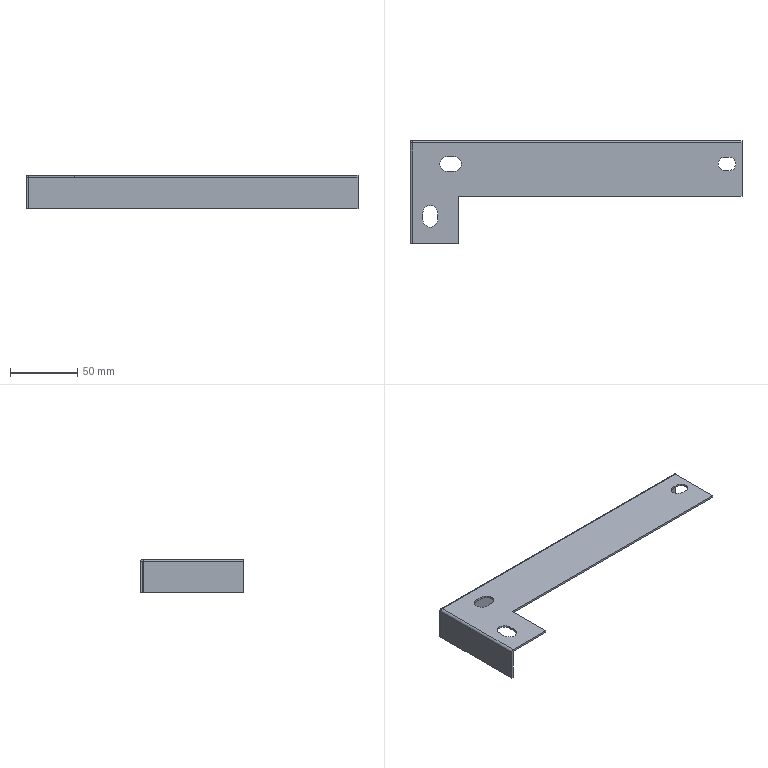Part | SolidWorks | features MirrorStock 1 | 1 solid | 39 faces | box 246 x 76 x 25 mm | volume 27497 mm3 | plane 27 | cylinder 12 | commonest cylinder face diameters 11 x5 10 x3 0.4 x2 3.4 x2
STEP:
#1=CARTESIAN_POINT('',(113.3,15.8,1.5));
#2=VERTEX_POINT('',#1);
#3=CARTESIAN_POINT('',(118.3,20.8,1.5));
#4=VERTEX_POINT('',#3);
#5=CARTESIAN_POINT('',(113.3,20.8,1.5));
#6=DIRECTION('',(0.,0.,1.));
#7=DIRECTION('',(1.,0.,0.));
#8=AXIS2_PLACEMENT_3D('',#5,#6,#7);
#9=CIRCLE('',#8,5.);
#10=EDGE_CURVE('',#2,#4,#9,.T.);
#11=ORIENTED_EDGE('',*,*,#10,.T.);
#12=CARTESIAN_POINT('',(118.3,20.8,0.));
#13=VERTEX_POINT('',#12);
#14=CARTESIAN_POINT('',(118.3,20.8,10.));
#15=DIRECTION('',(0.,0.,-1.));
#16=VECTOR('',#15,1000.);
#17=LINE('',#14,#16);
#18=EDGE_CURVE('',#4,#13,#17,.T.);
#19=ORIENTED_EDGE('',*,*,#18,.T.);
#20=CARTESIAN_POINT('',(113.3,15.8,0.));
#21=VERTEX_POINT('',#20);
#22=CARTESIAN_POINT('',(113.3,20.8,0.));
#23=DIRECTION('',(0.,0.,1.));
#24=DIRECTION('',(1.,0.,0.));
#25=AXIS2_PLACEMENT_3D('',#22,#23,#24);
#26=CIRCLE('',#25,5.);
#27=EDGE_CURVE('',#21,#13,#26,.T.);
#28=ORIENTED_EDGE('',*,*,#27,.F.);
#29=CARTESIAN_POINT('',(113.3,15.8,10.));
#30=DIRECTION('',(0.,0.,-1.));
#31=VECTOR('',#30,1000.);
#32=LINE('',#29,#31);
#33=EDGE_CURVE('',#2,#21,#32,.T.);
#34=ORIENTED_EDGE('',*,*,#33,.F.);
#35=EDGE_LOOP('',(#11,#19,#28,#34));
#36=FACE_OUTER_BOUND('',#35,.T.);
#37=CARTESIAN_POINT('',(113.3,20.8,10.));
#38=DIRECTION('',(0.,0.,-1.));
#39=DIRECTION('',(1.,0.,0.));
#40=AXIS2_PLACEMENT_3D('',#37,#38,#39);
#41=CYLINDRICAL_SURFACE('',#40,5.);
#42=ADVANCED_FACE('',(#36),#41,.F.);
#43=CARTESIAN_POINT('',(-90.5,15.3,1.5));
#44=VERTEX_POINT('',#43);
#45=CARTESIAN_POINT('',(-85.,20.8,1.5));
#46=VERTEX_POINT('',#45);
#47=CARTESIAN_POINT('',(-90.5,20.8,1.5));
#48=DIRECTION('',(0.,0.,1.));
#49=DIRECTION('',(1.,0.,0.));
#50=AXIS2_PLACEMENT_3D('',#47,#48,#49);
#51=CIRCLE('',#50,5.5);
#52=EDGE_CURVE('',#44,#46,#51,.T.);
#53=ORIENTED_EDGE('',*,*,#52,.T.);
#54=CARTESIAN_POINT('',(-85.,20.8,0.));
#55=VERTEX_POINT('',#54);
#56=CARTESIAN_POINT('',(-85.,20.8,10.));
#57=DIRECTION('',(0.,0.,-1.));
#58=VECTOR('',#57,1000.);
#59=LINE('',#56,#58);
#60=EDGE_CURVE('',#46,#55,#59,.T.);
#61=ORIENTED_EDGE('',*,*,#60,.T.);
#62=CARTESIAN_POINT('',(-90.5,15.3,0.));
#63=VERTEX_POINT('',#62);
#64=CARTESIAN_POINT('',(-90.5,20.8,0.));
#65=DIRECTION('',(0.,0.,1.));
#66=DIRECTION('',(1.,0.,0.));
#67=AXIS2_PLACEMENT_3D('',#64,#65,#66);
#68=CIRCLE('',#67,5.5);
#69=EDGE_CURVE('',#63,#55,#68,.T.);
#70=ORIENTED_EDGE('',*,*,#69,.F.);
#71=CARTESIAN_POINT('',(-90.5,15.3,10.));
#72=DIRECTION('',(0.,0.,-1.));
#73=VECTOR('',#72,1000.);
#74=LINE('',#71,#73);
#75=EDGE_CURVE('',#44,#63,#74,.T.);
#76=ORIENTED_EDGE('',*,*,#75,.F.);
#77=EDGE_LOOP('',(#53,#61,#70,#76));
#78=FACE_OUTER_BOUND('',#77,.T.);
#79=CARTESIAN_POINT('',(-90.5,20.8,10.));
#80=DIRECTION('',(0.,0.,-1.));
#81=DIRECTION('',(1.,0.,0.));
#82=AXIS2_PLACEMENT_3D('',#79,#80,#81);
#83=CYLINDRICAL_SURFACE('',#82,5.5);
#84=ADVANCED_FACE('',(#78),#83,.F.);
#85=CARTESIAN_POINT('',(-121.3,36.5,-0.2));
#86=VERTEX_POINT('',#85);
#87=CARTESIAN_POINT('',(-121.3,38.,-0.2));
#88=VERTEX_POINT('',#87);
#89=CARTESIAN_POINT('',(-121.3,36.5,-0.2));
#90=DIRECTION('',(0.,1.,0.));
#91=VECTOR('',#90,1000.);
#92=LINE('',#89,#91);
#93=EDGE_CURVE('',#86,#88,#92,.T.);
#94=ORIENTED_EDGE('',*,*,#93,.T.);
#95=CARTESIAN_POINT('',(-123.,38.,-0.2));
#96=VERTEX_POINT('',#95);
#97=CARTESIAN_POINT('',(123.,38.,-0.2));
#98=DIRECTION('',(1.,0.,0.));
#99=VECTOR('',#98,1000.);
#100=LINE('',#97,#99);
#101=EDGE_CURVE('',#96,#88,#100,.T.);
#102=ORIENTED_EDGE('',*,*,#101,.F.);
#103=CARTESIAN_POINT('',(-123.,36.5,-0.2));
#104=VERTEX_POINT('',#103);
#105=CARTESIAN_POINT('',(-123.,36.5,-0.2));
#106=DIRECTION('',(0.,1.,0.));
#107=VECTOR('',#106,1000.);
#108=LINE('',#105,#107);
#109=EDGE_CURVE('',#104,#96,#108,.T.);
#110=ORIENTED_EDGE('',*,*,#109,.F.);
#111=CARTESIAN_POINT('',(123.,36.5,-0.2));
#112=DIRECTION('',(-1.,0.,0.));
#113=VECTOR('',#112,1000.);
#114=LINE('',#111,#113);
#115=EDGE_CURVE('',#86,#104,#114,.T.);
#116=ORIENTED_EDGE('',*,*,#115,.F.);
#117=EDGE_LOOP('',(#94,#102,#110,#116));
#118=FACE_OUTER_BOUND('',#117,.T.);
#119=CARTESIAN_POINT('',(0.,0.,-0.2));
#120=DIRECTION('',(0.,0.,-1.));
#121=DIRECTION('',(0.,-1.,0.));
#122=AXIS2_PLACEMENT_3D('',#119,#120,#121);
#123=PLANE('',#122);
#124=ADVANCED_FACE('',(#118),#123,.F.);
#125=CARTESIAN_POINT('',(-121.3,36.3,1.5));
#126=VERTEX_POINT('',#125);
#127=CARTESIAN_POINT('',(123.,36.3,1.5));
#128=VERTEX_POINT('',#127);
#129=CARTESIAN_POINT('',(-123.,36.3,1.5));
#130=DIRECTION('',(1.,0.,0.));
#131=VECTOR('',#130,1000.);
#132=LINE('',#129,#131);
#133=EDGE_CURVE('',#126,#128,#132,.T.);
#134=ORIENTED_EDGE('',*,*,#133,.T.);
#135=CARTESIAN_POINT('',(123.,38.,-0.2));
#136=VERTEX_POINT('',#135);
#137=CARTESIAN_POINT('',(123.,36.3,-0.2));
#138=DIRECTION('',(-1.,0.,0.));
#139=DIRECTION('',(0.,0.,-1.));
#140=AXIS2_PLACEMENT_3D('',#137,#138,#139);
#141=CIRCLE('',#140,1.7);
#142=EDGE_CURVE('',#128,#136,#141,.T.);
#143=ORIENTED_EDGE('',*,*,#142,.T.);
#144=CARTESIAN_POINT('',(123.,38.,-0.2));
#145=DIRECTION('',(1.,0.,0.));
#146=VECTOR('',#145,1000.);
#147=LINE('',#144,#146);
#148=EDGE_CURVE('',#88,#136,#147,.T.);
#149=ORIENTED_EDGE('',*,*,#148,.F.);
#150=CARTESIAN_POINT('',(-121.3,36.3,-0.2));
#151=DIRECTION('',(-1.,0.,0.));
#152=DIRECTION('',(0.,0.,-1.));
#153=AXIS2_PLACEMENT_3D('',#150,#151,#152);
#154=CIRCLE('',#153,1.7);
#155=EDGE_CURVE('',#126,#88,#154,.T.);
#156=ORIENTED_EDGE('',*,*,#155,.F.);
#157=EDGE_LOOP('',(#134,#143,#149,#156));
#158=FACE_OUTER_BOUND('',#157,.T.);
#159=CARTESIAN_POINT('',(-123.,36.3,-0.2));
#160=DIRECTION('',(-1.,0.,0.));
#161=DIRECTION('',(0.,1.,0.));
#162=AXIS2_PLACEMENT_3D('',#159,#160,#161);
#163=CYLINDRICAL_SURFACE('',#162,1.7);
#164=ADVANCED_FACE('',(#158),#163,.T.);
#165=CARTESIAN_POINT('',(-121.3,36.3,0.));
#166=VERTEX_POINT('',#165);
#167=CARTESIAN_POINT('',(-121.3,36.3,-0.2));
#168=DIRECTION('',(-1.,0.,0.));
#169=DIRECTION('',(0.,0.,-1.));
#170=AXIS2_PLACEMENT_3D('',#167,#168,#169);
#171=CIRCLE('',#170,0.2);
#172=EDGE_CURVE('',#166,#86,#171,.T.);
#173=ORIENTED_EDGE('',*,*,#172,.F.);
#174=CARTESIAN_POINT('',(-121.3,36.3,0.));
#175=DIRECTION('',(0.,0.,1.));
#176=VECTOR('',#175,1000.);
#177=LINE('',#174,#176);
#178=EDGE_CURVE('',#166,#126,#177,.T.);
#179=ORIENTED_EDGE('',*,*,#178,.T.);
#180=ORIENTED_EDGE('',*,*,#155,.T.);
#181=ORIENTED_EDGE('',*,*,#93,.F.);
#182=EDGE_LOOP('',(#173,#179,#180,#181));
#183=FACE_OUTER_BOUND('',#182,.T.);
#184=CARTESIAN_POINT('',(-121.3,36.3,-0.2));
#185=DIRECTION('',(-1.,0.,0.));
#186=DIRECTION('',(0.,0.,-1.));
#187=AXIS2_PLACEMENT_3D('',#184,#185,#186);
#188=PLANE('',#187);
#189=ADVANCED_FACE('',(#183),#188,.T.);
#190=CARTESIAN_POINT('',(113.3,25.8,1.5));
#191=VERTEX_POINT('',#190);
#192=CARTESIAN_POINT('',(110.3,25.8,1.5));
#193=VERTEX_POINT('',#192);
#194=CARTESIAN_POINT('',(0.,25.8,1.5));
#195=DIRECTION('',(-1.,0.,0.));
#196=VECTOR('',#195,1000.);
#197=LINE('',#194,#196);
#198=EDGE_CURVE('',#191,#193,#197,.T.);
#199=ORIENTED_EDGE('',*,*,#198,.F.);
#200=CARTESIAN_POINT('',(113.3,20.8,1.5));
#201=DIRECTION('',(0.,0.,1.));
#202=DIRECTION('',(1.,0.,0.));
#203=AXIS2_PLACEMENT_3D('',#200,#201,#202);
#204=CIRCLE('',#203,5.);
#205=EDGE_CURVE('',#4,#191,#204,.T.);
#206=ORIENTED_EDGE('',*,*,#205,.F.);
#207=ORIENTED_EDGE('',*,*,#10,.F.);
#208=CARTESIAN_POINT('',(110.3,15.8,1.5));
#209=VERTEX_POINT('',#208);
#210=CARTESIAN_POINT('',(0.,15.8,1.5));
#211=DIRECTION('',(1.,0.,0.));
#212=VECTOR('',#211,1000.);
#213=LINE('',#210,#212);
#214=EDGE_CURVE('',#209,#2,#213,.T.);
#215=ORIENTED_EDGE('',*,*,#214,.F.);
#216=CARTESIAN_POINT('',(110.3,20.8,1.5));
#217=DIRECTION('',(0.,0.,1.));
#218=DIRECTION('',(1.,0.,0.));
#219=AXIS2_PLACEMENT_3D('',#216,#217,#218);
#220=CIRCLE('',#219,5.);
#221=EDGE_CURVE('',#193,#209,#220,.T.);
#222=ORIENTED_EDGE('',*,*,#221,.F.);
#223=EDGE_LOOP('',(#199,#206,#207,#215,#222));
#224=FACE_BOUND('',#223,.T.);
#225=CARTESIAN_POINT('',(-90.5,26.3,1.5));
#226=VERTEX_POINT('',#225);
#227=CARTESIAN_POINT('',(-95.5,26.3,1.5));
#228=VERTEX_POINT('',#227);
#229=CARTESIAN_POINT('',(0.,26.3,1.5));
#230=DIRECTION('',(-1.,0.,0.));
#231=VECTOR('',#230,1000.);
#232=LINE('',#229,#231);
#233=EDGE_CURVE('',#226,#228,#232,.T.);
#234=ORIENTED_EDGE('',*,*,#233,.F.);
#235=CARTESIAN_POINT('',(-90.5,20.8,1.5));
#236=DIRECTION('',(0.,0.,1.));
#237=DIRECTION('',(1.,0.,0.));
#238=AXIS2_PLACEMENT_3D('',#235,#236,#237);
#239=CIRCLE('',#238,5.5);
#240=EDGE_CURVE('',#46,#226,#239,.T.);
#241=ORIENTED_EDGE('',*,*,#240,.F.);
#242=ORIENTED_EDGE('',*,*,#52,.F.);
#243=CARTESIAN_POINT('',(-95.5,15.3,1.5));
#244=VERTEX_POINT('',#243);
#245=CARTESIAN_POINT('',(0.,15.3,1.5));
#246=DIRECTION('',(1.,0.,0.));
#247=VECTOR('',#246,1000.);
#248=LINE('',#245,#247);
#249=EDGE_CURVE('',#244,#44,#248,.T.);
#250=ORIENTED_EDGE('',*,*,#249,.F.);
#251=CARTESIAN_POINT('',(-95.5,20.8,1.5));
#252=DIRECTION('',(0.,0.,1.));
#253=DIRECTION('',(1.,0.,0.));
#254=AXIS2_PLACEMENT_3D('',#251,#252,#253);
#255=CIRCLE('',#254,5.5);
#256=EDGE_CURVE('',#228,#244,#255,.T.);
#257=ORIENTED_EDGE('',*,*,#256,.F.);
#258=EDGE_LOOP('',(#234,#241,#242,#250,#257));
#259=FACE_BOUND('',#258,.T.);
#260=CARTESIAN_POINT('',(-102.5,-20.5,1.5));
#261=VERTEX_POINT('',#260);
#262=CARTESIAN_POINT('',(-102.5,-15.5,1.5));
#263=VERTEX_POINT('',#262);
#264=CARTESIAN_POINT('',(-102.5,0.,1.5));
#265=DIRECTION('',(0.,1.,0.));
#266=VECTOR('',#265,1000.);
#267=LINE('',#264,#266);
#268=EDGE_CURVE('',#261,#263,#267,.T.);
#269=ORIENTED_EDGE('',*,*,#268,.F.);
#270=CARTESIAN_POINT('',(-113.5,-20.5,1.5));
#271=VERTEX_POINT('',#270);
#272=CARTESIAN_POINT('',(-108.,-20.5,1.5));
#273=DIRECTION('',(0.,0.,1.));
#274=DIRECTION('',(1.,0.,0.));
#275=AXIS2_PLACEMENT_3D('',#272,#273,#274);
#276=CIRCLE('',#275,5.5);
#277=EDGE_CURVE('',#271,#261,#276,.T.);
#278=ORIENTED_EDGE('',*,*,#277,.F.);
#279=CARTESIAN_POINT('',(-113.5,-15.5,1.5));
#280=VERTEX_POINT('',#279);
#281=CARTESIAN_POINT('',(-113.5,0.,1.5));
#282=DIRECTION('',(0.,-1.,0.));
#283=VECTOR('',#282,1000.);
#284=LINE('',#281,#283);
#285=EDGE_CURVE('',#280,#271,#284,.T.);
#286=ORIENTED_EDGE('',*,*,#285,.F.);
#287=CARTESIAN_POINT('',(-108.,-15.5,1.5));
#288=DIRECTION('',(0.,0.,1.));
#289=DIRECTION('',(1.,0.,0.));
#290=AXIS2_PLACEMENT_3D('',#287,#288,#289);
#291=CIRCLE('',#290,5.5);
#292=EDGE_CURVE('',#263,#280,#291,.T.);
#293=ORIENTED_EDGE('',*,*,#292,.F.);
#294=EDGE_LOOP('',(#269,#278,#286,#293));
#295=FACE_BOUND('',#294,.T.);
#296=CARTESIAN_POINT('',(123.,-3.,1.5));
#297=VERTEX_POINT('',#296);
#298=CARTESIAN_POINT('',(-87.,-3.,1.5));
#299=VERTEX_POINT('',#298);
#300=CARTESIAN_POINT('',(0.,-3.,1.5));
#301=DIRECTION('',(-1.,0.,0.));
#302=VECTOR('',#301,1000.);
#303=LINE('',#300,#302);
#304=EDGE_CURVE('',#297,#299,#303,.T.);
#305=ORIENTED_EDGE('',*,*,#304,.F.);
#306=CARTESIAN_POINT('',(123.,38.,1.5));
#307=DIRECTION('',(0.,1.,0.));
#308=VECTOR('',#307,1000.);
#309=LINE('',#306,#308);
#310=EDGE_CURVE('',#297,#128,#309,.T.);
#311=ORIENTED_EDGE('',*,*,#310,.T.);
#312=ORIENTED_EDGE('',*,*,#133,.F.);
#313=CARTESIAN_POINT('',(-121.3,-38.,1.5));
#314=VERTEX_POINT('',#313);
#315=CARTESIAN_POINT('',(-121.3,-38.,1.5));
#316=DIRECTION('',(0.,1.,0.));
#317=VECTOR('',#316,1000.);
#318=LINE('',#315,#317);
#319=EDGE_CURVE('',#314,#126,#318,.T.);
#320=ORIENTED_EDGE('',*,*,#319,.F.);
#321=CARTESIAN_POINT('',(-87.,-38.,1.5));
#322=VERTEX_POINT('',#321);
#323=CARTESIAN_POINT('',(-123.,-38.,1.5));
#324=DIRECTION('',(1.,0.,0.));
#325=VECTOR('',#324,1000.);
#326=LINE('',#323,#325);
#327=EDGE_CURVE('',#314,#322,#326,.T.);
#328=ORIENTED_EDGE('',*,*,#327,.T.);
#329=CARTESIAN_POINT('',(-87.,0.,1.5));
#330=DIRECTION('',(0.,-1.,0.));
#331=VECTOR('',#330,1000.);
#332=LINE('',#329,#331);
#333=EDGE_CURVE('',#299,#322,#332,.T.);
#334=ORIENTED_EDGE('',*,*,#333,.F.);
#335=EDGE_LOOP('',(#305,#311,#312,#320,#328,#334));
#336=FACE_OUTER_BOUND('',#335,.T.);
#337=CARTESIAN_POINT('',(0.,0.,1.5));
#338=DIRECTION('',(0.,0.,-1.));
#339=DIRECTION('',(1.,0.,0.));
#340=AXIS2_PLACEMENT_3D('',#337,#338,#339);
#341=PLANE('',#340);
#342=ADVANCED_FACE('',(#224,#259,#295,#336),#341,.F.);
#343=CARTESIAN_POINT('',(-87.,-3.,0.));
#344=VERTEX_POINT('',#343);
#345=CARTESIAN_POINT('',(-87.,-38.,0.));
#346=VERTEX_POINT('',#345);
#347=CARTESIAN_POINT('',(-87.,-38.,0.));
#348=DIRECTION('',(0.,-1.,0.));
#349=VECTOR('',#348,1000.);
#350=LINE('',#347,#349);
#351=EDGE_CURVE('',#344,#346,#350,.T.);
#352=ORIENTED_EDGE('',*,*,#351,.T.);
#353=CARTESIAN_POINT('',(-121.3,-38.,0.));
#354=VERTEX_POINT('',#353);
#355=CARTESIAN_POINT('',(-123.,-38.,0.));
#356=DIRECTION('',(1.,0.,0.));
#357=VECTOR('',#356,1000.);
#358=LINE('',#355,#357);
#359=EDGE_CURVE('',#354,#346,#358,.T.);
#360=ORIENTED_EDGE('',*,*,#359,.F.);
#361=CARTESIAN_POINT('',(-121.3,-38.,0.));
#362=DIRECTION('',(0.,1.,0.));
#363=VECTOR('',#362,1000.);
#364=LINE('',#361,#363);
#365=EDGE_CURVE('',#354,#166,#364,.T.);
#366=ORIENTED_EDGE('',*,*,#365,.T.);
#367=CARTESIAN_POINT('',(123.,36.3,0.));
#368=VERTEX_POINT('',#367);
#369=CARTESIAN_POINT('',(-123.,36.3,0.));
#370=DIRECTION('',(1.,0.,0.));
#371=VECTOR('',#370,1000.);
#372=LINE('',#369,#371);
#373=EDGE_CURVE('',#166,#368,#372,.T.);
#374=ORIENTED_EDGE('',*,*,#373,.T.);
#375=CARTESIAN_POINT('',(123.,-3.,0.));
#376=VERTEX_POINT('',#375);
#377=CARTESIAN_POINT('',(123.,38.,0.));
#378=DIRECTION('',(0.,1.,0.));
#379=VECTOR('',#378,1000.);
#380=LINE('',#377,#379);
#381=EDGE_CURVE('',#376,#368,#380,.T.);
#382=ORIENTED_EDGE('',*,*,#381,.F.);
#383=CARTESIAN_POINT('',(123.,-3.,0.));
#384=DIRECTION('',(-1.,0.,0.));
#385=VECTOR('',#384,1000.);
#386=LINE('',#383,#385);
#387=EDGE_CURVE('',#376,#344,#386,.T.);
#388=ORIENTED_EDGE('',*,*,#387,.T.);
#389=EDGE_LOOP('',(#352,#360,#366,#374,#382,#388));
#390=FACE_OUTER_BOUND('',#389,.T.);
#391=CARTESIAN_POINT('',(110.3,25.8,0.));
#392=VERTEX_POINT('',#391);
#393=CARTESIAN_POINT('',(110.3,15.8,0.));
#394=VERTEX_POINT('',#393);
#395=CARTESIAN_POINT('',(110.3,20.8,0.));
#396=DIRECTION('',(0.,0.,1.));
#397=DIRECTION('',(1.,0.,0.));
#398=AXIS2_PLACEMENT_3D('',#395,#396,#397);
#399=CIRCLE('',#398,5.);
#400=EDGE_CURVE('',#392,#394,#399,.T.);
#401=ORIENTED_EDGE('',*,*,#400,.T.);
#402=CARTESIAN_POINT('',(110.3,15.8,0.));
#403=DIRECTION('',(1.,0.,0.));
#404=VECTOR('',#403,1000.);
#405=LINE('',#402,#404);
#406=EDGE_CURVE('',#394,#21,#405,.T.);
#407=ORIENTED_EDGE('',*,*,#406,.T.);
#408=ORIENTED_EDGE('',*,*,#27,.T.);
#409=CARTESIAN_POINT('',(113.3,25.8,0.));
#410=VERTEX_POINT('',#409);
#411=CARTESIAN_POINT('',(113.3,20.8,0.));
#412=DIRECTION('',(0.,0.,1.));
#413=DIRECTION('',(1.,0.,0.));
#414=AXIS2_PLACEMENT_3D('',#411,#412,#413);
#415=CIRCLE('',#414,5.);
#416=EDGE_CURVE('',#13,#410,#415,.T.);
#417=ORIENTED_EDGE('',*,*,#416,.T.);
#418=CARTESIAN_POINT('',(110.3,25.8,0.));
#419=DIRECTION('',(-1.,0.,0.));
#420=VECTOR('',#419,1000.);
#421=LINE('',#418,#420);
#422=EDGE_CURVE('',#410,#392,#421,.T.);
#423=ORIENTED_EDGE('',*,*,#422,.T.);
#424=EDGE_LOOP('',(#401,#407,#408,#417,#423));
#425=FACE_BOUND('',#424,.T.);
#426=CARTESIAN_POINT('',(-95.5,26.3,0.));
#427=VERTEX_POINT('',#426);
#428=CARTESIAN_POINT('',(-95.5,15.3,0.));
#429=VERTEX_POINT('',#428);
#430=CARTESIAN_POINT('',(-95.5,20.8,0.));
#431=DIRECTION('',(0.,0.,1.));
#432=DIRECTION('',(1.,0.,0.));
#433=AXIS2_PLACEMENT_3D('',#430,#431,#432);
#434=CIRCLE('',#433,5.5);
#435=EDGE_CURVE('',#427,#429,#434,.T.);
#436=ORIENTED_EDGE('',*,*,#435,.T.);
#437=CARTESIAN_POINT('',(-95.5,15.3,0.));
#438=DIRECTION('',(1.,0.,0.));
#439=VECTOR('',#438,1000.);
#440=LINE('',#437,#439);
#441=EDGE_CURVE('',#429,#63,#440,.T.);
#442=ORIENTED_EDGE('',*,*,#441,.T.);
#443=ORIENTED_EDGE('',*,*,#69,.T.);
#444=CARTESIAN_POINT('',(-90.5,26.3,0.));
#445=VERTEX_POINT('',#444);
#446=CARTESIAN_POINT('',(-90.5,20.8,0.));
#447=DIRECTION('',(0.,0.,1.));
#448=DIRECTION('',(1.,0.,0.));
#449=AXIS2_PLACEMENT_3D('',#446,#447,#448);
#450=CIRCLE('',#449,5.5);
#451=EDGE_CURVE('',#55,#445,#450,.T.);
#452=ORIENTED_EDGE('',*,*,#451,.T.);
#453=CARTESIAN_POINT('',(-95.5,26.3,0.));
#454=DIRECTION('',(-1.,0.,0.));
#455=VECTOR('',#454,1000.);
#456=LINE('',#453,#455);
#457=EDGE_CURVE('',#445,#427,#456,.T.);
#458=ORIENTED_EDGE('',*,*,#457,.T.);
#459=EDGE_LOOP('',(#436,#442,#443,#452,#458));
#460=FACE_BOUND('',#459,.T.);
#461=CARTESIAN_POINT('',(-102.5,-15.5,0.));
#462=VERTEX_POINT('',#461);
#463=CARTESIAN_POINT('',(-113.5,-15.5,0.));
#464=VERTEX_POINT('',#463);
#465=CARTESIAN_POINT('',(-108.,-15.5,0.));
#466=DIRECTION('',(0.,0.,1.));
#467=DIRECTION('',(1.,0.,0.));
#468=AXIS2_PLACEMENT_3D('',#465,#466,#467);
#469=CIRCLE('',#468,5.5);
#470=EDGE_CURVE('',#462,#464,#469,.T.);
#471=ORIENTED_EDGE('',*,*,#470,.T.);
#472=CARTESIAN_POINT('',(-113.5,-20.5,0.));
#473=VERTEX_POINT('',#472);
#474=CARTESIAN_POINT('',(-113.5,-15.5,0.));
#475=DIRECTION('',(0.,-1.,0.));
#476=VECTOR('',#475,1000.);
#477=LINE('',#474,#476);
#478=EDGE_CURVE('',#464,#473,#477,.T.);
#479=ORIENTED_EDGE('',*,*,#478,.T.);
#480=CARTESIAN_POINT('',(-102.5,-20.5,0.));
#481=VERTEX_POINT('',#480);
#482=CARTESIAN_POINT('',(-108.,-20.5,0.));
#483=DIRECTION('',(0.,0.,1.));
#484=DIRECTION('',(1.,0.,0.));
#485=AXIS2_PLACEMENT_3D('',#482,#483,#484);
#486=CIRCLE('',#485,5.5);
#487=EDGE_CURVE('',#473,#481,#486,.T.);
#488=ORIENTED_EDGE('',*,*,#487,.T.);
#489=CARTESIAN_POINT('',(-102.5,-15.5,0.));
#490=DIRECTION('',(0.,1.,0.));
#491=VECTOR('',#490,1000.);
#492=LINE('',#489,#491);
#493=EDGE_CURVE('',#481,#462,#492,.T.);
#494=ORIENTED_EDGE('',*,*,#493,.T.);
#495=EDGE_LOOP('',(#471,#479,#488,#494));
#496=FACE_BOUND('',#495,.T.);
#497=CARTESIAN_POINT('',(0.,0.,0.));
#498=DIRECTION('',(0.,0.,-1.));
#499=DIRECTION('',(1.,0.,0.));
#500=AXIS2_PLACEMENT_3D('',#497,#498,#499);
#501=PLANE('',#500);
#502=ADVANCED_FACE('',(#390,#425,#460,#496),#501,.T.);
#503=CARTESIAN_POINT('',(-87.,-38.,10.));
#504=DIRECTION('',(0.,0.,-1.));
#505=VECTOR('',#504,1000.);
#506=LINE('',#503,#505);
#507=EDGE_CURVE('',#322,#346,#506,.T.);
#508=ORIENTED_EDGE('',*,*,#507,.F.);
#509=ORIENTED_EDGE('',*,*,#327,.F.);
#510=CARTESIAN_POINT('',(-121.3,-38.,0.));
#511=DIRECTION('',(0.,0.,1.));
#512=VECTOR('',#511,1000.);
#513=LINE('',#510,#512);
#514=EDGE_CURVE('',#354,#314,#513,.T.);
#515=ORIENTED_EDGE('',*,*,#514,.F.);
#516=ORIENTED_EDGE('',*,*,#359,.T.);
#517=EDGE_LOOP('',(#508,#509,#515,#516));
#518=FACE_OUTER_BOUND('',#517,.T.);
#519=CARTESIAN_POINT('',(-123.,-38.,1.5));
#520=DIRECTION('',(0.,-1.,0.));
#521=DIRECTION('',(0.,0.,1.));
#522=AXIS2_PLACEMENT_3D('',#519,#520,#521);
#523=PLANE('',#522);
#524=ADVANCED_FACE('',(#518),#523,.T.);
#525=CARTESIAN_POINT('',(123.,-3.,1.5));
#526=DIRECTION('',(0.,0.,-1.));
#527=VECTOR('',#526,1000.);
#528=LINE('',#525,#527);
#529=EDGE_CURVE('',#297,#376,#528,.T.);
#530=ORIENTED_EDGE('',*,*,#529,.T.);
#531=ORIENTED_EDGE('',*,*,#381,.T.);
#532=CARTESIAN_POINT('',(123.,36.3,0.));
#533=DIRECTION('',(0.,0.,1.));
#534=VECTOR('',#533,1000.);
#535=LINE('',#532,#534);
#536=EDGE_CURVE('',#368,#128,#535,.T.);
#537=ORIENTED_EDGE('',*,*,#536,.T.);
#538=ORIENTED_EDGE('',*,*,#310,.F.);
#539=EDGE_LOOP('',(#530,#531,#537,#538));
#540=FACE_OUTER_BOUND('',#539,.T.);
#541=CARTESIAN_POINT('',(123.,38.,1.5));
#542=DIRECTION('',(1.,0.,0.));
#543=DIRECTION('',(0.,0.,1.));
#544=AXIS2_PLACEMENT_3D('',#541,#542,#543);
#545=PLANE('',#544);
#546=ADVANCED_FACE('',(#540),#545,.T.);
#547=CARTESIAN_POINT('',(123.,36.5,-0.2));
#548=VERTEX_POINT('',#547);
#549=CARTESIAN_POINT('',(123.,38.,-0.2));
#550=DIRECTION('',(0.,1.,0.));
#551=VECTOR('',#550,1000.);
#552=LINE('',#549,#551);
#553=EDGE_CURVE('',#548,#136,#552,.T.);
#554=ORIENTED_EDGE('',*,*,#553,.T.);
#555=ORIENTED_EDGE('',*,*,#142,.F.);
#556=ORIENTED_EDGE('',*,*,#536,.F.);
#557=CARTESIAN_POINT('',(123.,36.3,-0.2));
#558=DIRECTION('',(-1.,0.,0.));
#559=DIRECTION('',(0.,0.,-1.));
#560=AXIS2_PLACEMENT_3D('',#557,#558,#559);
#561=CIRCLE('',#560,0.2);
#562=EDGE_CURVE('',#368,#548,#561,.T.);
#563=ORIENTED_EDGE('',*,*,#562,.T.);
#564=EDGE_LOOP('',(#554,#555,#556,#563));
#565=FACE_OUTER_BOUND('',#564,.T.);
#566=CARTESIAN_POINT('',(123.,36.3,-0.2));
#567=DIRECTION('',(1.,0.,0.));
#568=DIRECTION('',(0.,0.,1.));
#569=AXIS2_PLACEMENT_3D('',#566,#567,#568);
#570=PLANE('',#569);
#571=ADVANCED_FACE('',(#565),#570,.T.);
#572=ORIENTED_EDGE('',*,*,#172,.T.);
#573=CARTESIAN_POINT('',(123.,36.5,-0.2));
#574=DIRECTION('',(-1.,0.,0.));
#575=VECTOR('',#574,1000.);
#576=LINE('',#573,#575);
#577=EDGE_CURVE('',#548,#86,#576,.T.);
#578=ORIENTED_EDGE('',*,*,#577,.F.);
#579=ORIENTED_EDGE('',*,*,#562,.F.);
#580=ORIENTED_EDGE('',*,*,#373,.F.);
#581=EDGE_LOOP('',(#572,#578,#579,#580));
#582=FACE_OUTER_BOUND('',#581,.T.);
#583=CARTESIAN_POINT('',(-123.,36.3,-0.2));
#584=DIRECTION('',(-1.,0.,0.));
#585=DIRECTION('',(0.,1.,0.));
#586=AXIS2_PLACEMENT_3D('',#583,#584,#585);
#587=CYLINDRICAL_SURFACE('',#586,0.2);
#588=ADVANCED_FACE('',(#582),#587,.F.);
#589=ORIENTED_EDGE('',*,*,#553,.F.);
#590=CARTESIAN_POINT('',(123.,36.5,-23.5));
#591=VERTEX_POINT('',#590);
#592=CARTESIAN_POINT('',(123.,36.5,0.));
#593=DIRECTION('',(0.,0.,1.));
#594=VECTOR('',#593,1000.);
#595=LINE('',#592,#594);
#596=EDGE_CURVE('',#591,#548,#595,.T.);
#597=ORIENTED_EDGE('',*,*,#596,.F.);
#598=CARTESIAN_POINT('',(123.,38.,-23.5));
#599=VERTEX_POINT('',#598);
#600=CARTESIAN_POINT('',(123.,38.,-23.5));
#601=DIRECTION('',(0.,-1.,0.));
#602=VECTOR('',#601,1000.);
#603=LINE('',#600,#602);
#604=EDGE_CURVE('',#599,#591,#603,.T.);
#605=ORIENTED_EDGE('',*,*,#604,.F.);
#606=CARTESIAN_POINT('',(123.,38.,0.));
#607=DIRECTION('',(0.,0.,1.));
#608=VECTOR('',#607,1000.);
#609=LINE('',#606,#608);
#610=EDGE_CURVE('',#599,#136,#609,.T.);
#611=ORIENTED_EDGE('',*,*,#610,.T.);
#612=EDGE_LOOP('',(#589,#597,#605,#611));
#613=FACE_OUTER_BOUND('',#612,.T.);
#614=CARTESIAN_POINT('',(123.,38.,0.));
#615=DIRECTION('',(-1.,0.,0.));
#616=DIRECTION('',(0.,0.,-1.));
#617=AXIS2_PLACEMENT_3D('',#614,#615,#616);
#618=PLANE('',#617);
#619=ADVANCED_FACE('',(#613),#618,.F.);
#620=ORIENTED_EDGE('',*,*,#109,.T.);
#621=CARTESIAN_POINT('',(-123.,38.,-23.5));
#622=VERTEX_POINT('',#621);
#623=CARTESIAN_POINT('',(-123.,38.,0.));
#624=DIRECTION('',(0.,0.,-1.));
#625=VECTOR('',#624,1000.);
#626=LINE('',#623,#625);
#627=EDGE_CURVE('',#96,#622,#626,.T.);
#628=ORIENTED_EDGE('',*,*,#627,.T.);
#629=CARTESIAN_POINT('',(-123.,36.5,-23.5));
#630=VERTEX_POINT('',#629);
#631=CARTESIAN_POINT('',(-123.,38.,-23.5));
#632=DIRECTION('',(0.,-1.,0.));
#633=VECTOR('',#632,1000.);
#634=LINE('',#631,#633);
#635=EDGE_CURVE('',#622,#630,#634,.T.);
#636=ORIENTED_EDGE('',*,*,#635,.T.);
#637=CARTESIAN_POINT('',(-123.,36.5,-23.5));
#638=DIRECTION('',(0.,0.,-1.));
#639=VECTOR('',#638,1000.);
#640=LINE('',#637,#639);
#641=EDGE_CURVE('',#104,#630,#640,.T.);
#642=ORIENTED_EDGE('',*,*,#641,.F.);
#643=EDGE_LOOP('',(#620,#628,#636,#642));
#644=FACE_OUTER_BOUND('',#643,.T.);
#645=CARTESIAN_POINT('',(-123.,38.,-23.5));
#646=DIRECTION('',(1.,0.,0.));
#647=DIRECTION('',(0.,0.,1.));
#648=AXIS2_PLACEMENT_3D('',#645,#646,#647);
#649=PLANE('',#648);
#650=ADVANCED_FACE('',(#644),#649,.F.);
#651=ORIENTED_EDGE('',*,*,#101,.T.);
#652=ORIENTED_EDGE('',*,*,#148,.T.);
#653=ORIENTED_EDGE('',*,*,#610,.F.);
#654=CARTESIAN_POINT('',(0.,38.,-23.5));
#655=DIRECTION('',(1.,0.,0.));
#656=VECTOR('',#655,1000.);
#657=LINE('',#654,#656);
#658=EDGE_CURVE('',#622,#599,#657,.T.);
#659=ORIENTED_EDGE('',*,*,#658,.F.);
#660=ORIENTED_EDGE('',*,*,#627,.F.);
#661=EDGE_LOOP('',(#651,#652,#653,#659,#660));
#662=FACE_OUTER_BOUND('',#661,.T.);
#663=CARTESIAN_POINT('',(0.,38.,0.));
#664=DIRECTION('',(0.,-1.,0.));
#665=DIRECTION('',(0.,0.,1.));
#666=AXIS2_PLACEMENT_3D('',#663,#664,#665);
#667=PLANE('',#666);
#668=ADVANCED_FACE('',(#662),#667,.F.);
#669=ORIENTED_EDGE('',*,*,#641,.T.);
#670=CARTESIAN_POINT('',(123.,36.5,-23.5));
#671=DIRECTION('',(1.,0.,0.));
#672=VECTOR('',#671,1000.);
#673=LINE('',#670,#672);
#674=EDGE_CURVE('',#630,#591,#673,.T.);
#675=ORIENTED_EDGE('',*,*,#674,.T.);
#676=ORIENTED_EDGE('',*,*,#596,.T.);
#677=ORIENTED_EDGE('',*,*,#577,.T.);
#678=ORIENTED_EDGE('',*,*,#115,.T.);
#679=EDGE_LOOP('',(#669,#675,#676,#677,#678));
#680=FACE_OUTER_BOUND('',#679,.T.);
#681=CARTESIAN_POINT('',(0.,36.5,0.));
#682=DIRECTION('',(0.,-1.,0.));
#683=DIRECTION('',(0.,0.,1.));
#684=AXIS2_PLACEMENT_3D('',#681,#682,#683);
#685=PLANE('',#684);
#686=ADVANCED_FACE('',(#680),#685,.T.);
#687=ORIENTED_EDGE('',*,*,#674,.F.);
#688=ORIENTED_EDGE('',*,*,#635,.F.);
#689=ORIENTED_EDGE('',*,*,#658,.T.);
#690=ORIENTED_EDGE('',*,*,#604,.T.);
#691=EDGE_LOOP('',(#687,#688,#689,#690));
#692=FACE_OUTER_BOUND('',#691,.T.);
#693=CARTESIAN_POINT('',(123.,38.,-23.5));
#694=DIRECTION('',(0.,0.,1.));
#695=DIRECTION('',(0.,1.,0.));
#696=AXIS2_PLACEMENT_3D('',#693,#694,#695);
#697=PLANE('',#696);
#698=ADVANCED_FACE('',(#692),#697,.F.);
#699=CARTESIAN_POINT('',(-121.5,36.3,-0.2));
#700=VERTEX_POINT('',#699);
#701=CARTESIAN_POINT('',(-123.,36.3,-0.2));
#702=VERTEX_POINT('',#701);
#703=CARTESIAN_POINT('',(-123.,36.3,-0.2));
#704=DIRECTION('',(-1.,0.,0.));
#705=VECTOR('',#704,1000.);
#706=LINE('',#703,#705);
#707=EDGE_CURVE('',#700,#702,#706,.T.);
#708=ORIENTED_EDGE('',*,*,#707,.T.);
#709=CARTESIAN_POINT('',(-121.3,36.3,-0.2));
#710=DIRECTION('',(0.,-1.,0.));
#711=DIRECTION('',(0.,0.,1.));
#712=AXIS2_PLACEMENT_3D('',#709,#710,#711);
#713=CIRCLE('',#712,1.7);
#714=EDGE_CURVE('',#126,#702,#713,.T.);
#715=ORIENTED_EDGE('',*,*,#714,.F.);
#716=ORIENTED_EDGE('',*,*,#178,.F.);
#717=CARTESIAN_POINT('',(-121.3,36.3,-0.2));
#718=DIRECTION('',(0.,-1.,0.));
#719=DIRECTION('',(0.,0.,1.));
#720=AXIS2_PLACEMENT_3D('',#717,#718,#719);
#721=CIRCLE('',#720,0.2);
#722=EDGE_CURVE('',#166,#700,#721,.T.);
#723=ORIENTED_EDGE('',*,*,#722,.T.);
#724=EDGE_LOOP('',(#708,#715,#716,#723));
#725=FACE_OUTER_BOUND('',#724,.T.);
#726=CARTESIAN_POINT('',(-121.3,36.3,-0.2));
#727=DIRECTION('',(0.,1.,0.));
#728=DIRECTION('',(0.,0.,-1.));
#729=AXIS2_PLACEMENT_3D('',#726,#727,#728);
#730=PLANE('',#729);
#731=ADVANCED_FACE('',(#725),#730,.T.);
#732=CARTESIAN_POINT('',(-121.5,-38.,-0.2));
#733=VERTEX_POINT('',#732);
#734=CARTESIAN_POINT('',(-121.3,-38.,-0.2));
#735=DIRECTION('',(0.,1.,0.));
#736=DIRECTION('',(0.,0.,1.));
#737=AXIS2_PLACEMENT_3D('',#734,#735,#736);
#738=CIRCLE('',#737,0.2);
#739=EDGE_CURVE('',#733,#354,#738,.T.);
#740=ORIENTED_EDGE('',*,*,#739,.T.);
#741=ORIENTED_EDGE('',*,*,#514,.T.);
#742=CARTESIAN_POINT('',(-123.,-38.,-0.2));
#743=VERTEX_POINT('',#742);
#744=CARTESIAN_POINT('',(-121.3,-38.,-0.2));
#745=DIRECTION('',(0.,1.,0.));
#746=DIRECTION('',(0.,0.,1.));
#747=AXIS2_PLACEMENT_3D('',#744,#745,#746);
#748=CIRCLE('',#747,1.7);
#749=EDGE_CURVE('',#743,#314,#748,.T.);
#750=ORIENTED_EDGE('',*,*,#749,.F.);
#751=CARTESIAN_POINT('',(-121.5,-38.,-0.2));
#752=DIRECTION('',(-1.,0.,0.));
#753=VECTOR('',#752,1000.);
#754=LINE('',#751,#753);
#755=EDGE_CURVE('',#733,#743,#754,.T.);
#756=ORIENTED_EDGE('',*,*,#755,.F.);
#757=EDGE_LOOP('',(#740,#741,#750,#756));
#758=FACE_OUTER_BOUND('',#757,.T.);
#759=CARTESIAN_POINT('',(-121.3,-38.,-0.2));
#760=DIRECTION('',(0.,1.,0.));
#761=DIRECTION('',(0.,0.,-1.));
#762=AXIS2_PLACEMENT_3D('',#759,#760,#761);
#763=PLANE('',#762);
#764=ADVANCED_FACE('',(#758),#763,.F.);
#765=ORIENTED_EDGE('',*,*,#319,.T.);
#766=ORIENTED_EDGE('',*,*,#714,.T.);
#767=CARTESIAN_POINT('',(-123.,0.,-0.2));
#768=DIRECTION('',(0.,-1.,0.));
#769=VECTOR('',#768,1000.);
#770=LINE('',#767,#769);
#771=EDGE_CURVE('',#702,#743,#770,.T.);
#772=ORIENTED_EDGE('',*,*,#771,.T.);
#773=ORIENTED_EDGE('',*,*,#749,.T.);
#774=EDGE_LOOP('',(#765,#766,#772,#773));
#775=FACE_OUTER_BOUND('',#774,.T.);
#776=CARTESIAN_POINT('',(-121.3,-38.,-0.2));
#777=DIRECTION('',(0.,-1.,0.));
#778=DIRECTION('',(-1.,0.,0.));
#779=AXIS2_PLACEMENT_3D('',#776,#777,#778);
#780=CYLINDRICAL_SURFACE('',#779,1.7);
#781=ADVANCED_FACE('',(#775),#780,.T.);
#782=ORIENTED_EDGE('',*,*,#365,.F.);
#783=ORIENTED_EDGE('',*,*,#739,.F.);
#784=CARTESIAN_POINT('',(-121.5,36.3,-0.2));
#785=DIRECTION('',(0.,-1.,0.));
#786=VECTOR('',#785,1000.);
#787=LINE('',#784,#786);
#788=EDGE_CURVE('',#700,#733,#787,.T.);
#789=ORIENTED_EDGE('',*,*,#788,.F.);
#790=ORIENTED_EDGE('',*,*,#722,.F.);
#791=EDGE_LOOP('',(#782,#783,#789,#790));
#792=FACE_OUTER_BOUND('',#791,.T.);
#793=CARTESIAN_POINT('',(-121.3,-38.,-0.2));
#794=DIRECTION('',(0.,-1.,0.));
#795=DIRECTION('',(-1.,0.,0.));
#796=AXIS2_PLACEMENT_3D('',#793,#794,#795);
#797=CYLINDRICAL_SURFACE('',#796,0.2);
#798=ADVANCED_FACE('',(#792),#797,.F.);
#799=CARTESIAN_POINT('',(-123.,-38.,-23.5));
#800=VERTEX_POINT('',#799);
#801=CARTESIAN_POINT('',(-123.,-38.,0.));
#802=DIRECTION('',(0.,0.,1.));
#803=VECTOR('',#802,1000.);
#804=LINE('',#801,#803);
#805=EDGE_CURVE('',#800,#743,#804,.T.);
#806=ORIENTED_EDGE('',*,*,#805,.F.);
#807=CARTESIAN_POINT('',(-121.5,-38.,-23.5));
#808=VERTEX_POINT('',#807);
#809=CARTESIAN_POINT('',(-123.,-38.,-23.5));
#810=DIRECTION('',(1.,0.,0.));
#811=VECTOR('',#810,1000.);
#812=LINE('',#809,#811);
#813=EDGE_CURVE('',#800,#808,#812,.T.);
#814=ORIENTED_EDGE('',*,*,#813,.T.);
#815=CARTESIAN_POINT('',(-121.5,-38.,0.));
#816=DIRECTION('',(0.,0.,1.));
#817=VECTOR('',#816,1000.);
#818=LINE('',#815,#817);
#819=EDGE_CURVE('',#808,#733,#818,.T.);
#820=ORIENTED_EDGE('',*,*,#819,.T.);
#821=ORIENTED_EDGE('',*,*,#755,.T.);
#822=EDGE_LOOP('',(#806,#814,#820,#821));
#823=FACE_OUTER_BOUND('',#822,.T.);
#824=CARTESIAN_POINT('',(-123.,-38.,0.));
#825=DIRECTION('',(0.,-1.,0.));
#826=DIRECTION('',(0.,0.,1.));
#827=AXIS2_PLACEMENT_3D('',#824,#825,#826);
#828=PLANE('',#827);
#829=ADVANCED_FACE('',(#823),#828,.T.);
#830=CARTESIAN_POINT('',(-121.5,36.3,-23.5));
#831=VERTEX_POINT('',#830);
#832=CARTESIAN_POINT('',(-121.5,36.3,0.));
#833=DIRECTION('',(0.,0.,-1.));
#834=VECTOR('',#833,1000.);
#835=LINE('',#832,#834);
#836=EDGE_CURVE('',#700,#831,#835,.T.);
#837=ORIENTED_EDGE('',*,*,#836,.T.);
#838=CARTESIAN_POINT('',(-123.,36.3,-23.5));
#839=VERTEX_POINT('',#838);
#840=CARTESIAN_POINT('',(-123.,36.3,-23.5));
#841=DIRECTION('',(1.,0.,0.));
#842=VECTOR('',#841,1000.);
#843=LINE('',#840,#842);
#844=EDGE_CURVE('',#839,#831,#843,.T.);
#845=ORIENTED_EDGE('',*,*,#844,.F.);
#846=CARTESIAN_POINT('',(-123.,36.3,-23.5));
#847=DIRECTION('',(0.,0.,-1.));
#848=VECTOR('',#847,1000.);
#849=LINE('',#846,#848);
#850=EDGE_CURVE('',#702,#839,#849,.T.);
#851=ORIENTED_EDGE('',*,*,#850,.F.);
#852=ORIENTED_EDGE('',*,*,#707,.F.);
#853=EDGE_LOOP('',(#837,#845,#851,#852));
#854=FACE_OUTER_BOUND('',#853,.T.);
#855=CARTESIAN_POINT('',(-123.,36.3,-23.5));
#856=DIRECTION('',(0.,1.,0.));
#857=DIRECTION('',(0.,0.,-1.));
#858=AXIS2_PLACEMENT_3D('',#855,#856,#857);
#859=PLANE('',#858);
#860=ADVANCED_FACE('',(#854),#859,.T.);
#861=ORIENTED_EDGE('',*,*,#850,.T.);
#862=CARTESIAN_POINT('',(-123.,-38.,-23.5));
#863=DIRECTION('',(0.,-1.,0.));
#864=VECTOR('',#863,1000.);
#865=LINE('',#862,#864);
#866=EDGE_CURVE('',#839,#800,#865,.T.);
#867=ORIENTED_EDGE('',*,*,#866,.T.);
#868=ORIENTED_EDGE('',*,*,#805,.T.);
#869=ORIENTED_EDGE('',*,*,#771,.F.);
#870=EDGE_LOOP('',(#861,#867,#868,#869));
#871=FACE_OUTER_BOUND('',#870,.T.);
#872=CARTESIAN_POINT('',(-123.,0.,0.));
#873=DIRECTION('',(-1.,0.,0.));
#874=DIRECTION('',(0.,0.,-1.));
#875=AXIS2_PLACEMENT_3D('',#872,#873,#874);
#876=PLANE('',#875);
#877=ADVANCED_FACE('',(#871),#876,.T.);
#878=ORIENTED_EDGE('',*,*,#788,.T.);
#879=ORIENTED_EDGE('',*,*,#819,.F.);
#880=CARTESIAN_POINT('',(-121.5,0.,-23.5));
#881=DIRECTION('',(0.,-1.,0.));
#882=VECTOR('',#881,1000.);
#883=LINE('',#880,#882);
#884=EDGE_CURVE('',#831,#808,#883,.T.);
#885=ORIENTED_EDGE('',*,*,#884,.F.);
#886=ORIENTED_EDGE('',*,*,#836,.F.);
#887=EDGE_LOOP('',(#878,#879,#885,#886));
#888=FACE_OUTER_BOUND('',#887,.T.);
#889=CARTESIAN_POINT('',(-121.5,0.,0.));
#890=DIRECTION('',(-1.,0.,0.));
#891=DIRECTION('',(0.,0.,-1.));
#892=AXIS2_PLACEMENT_3D('',#889,#890,#891);
#893=PLANE('',#892);
#894=ADVANCED_FACE('',(#888),#893,.F.);
#895=ORIENTED_EDGE('',*,*,#884,.T.);
#896=ORIENTED_EDGE('',*,*,#813,.F.);
#897=ORIENTED_EDGE('',*,*,#866,.F.);
#898=ORIENTED_EDGE('',*,*,#844,.T.);
#899=EDGE_LOOP('',(#895,#896,#897,#898));
#900=FACE_OUTER_BOUND('',#899,.T.);
#901=CARTESIAN_POINT('',(-123.,-38.,-23.5));
#902=DIRECTION('',(0.,0.,-1.));
#903=DIRECTION('',(1.,0.,0.));
#904=AXIS2_PLACEMENT_3D('',#901,#902,#903);
#905=PLANE('',#904);
#906=ADVANCED_FACE('',(#900),#905,.T.);
#907=CARTESIAN_POINT('',(-102.5,-15.5,10.));
#908=DIRECTION('',(0.,0.,-1.));
#909=VECTOR('',#908,1000.);
#910=LINE('',#907,#909);
#911=EDGE_CURVE('',#263,#462,#910,.T.);
#912=ORIENTED_EDGE('',*,*,#911,.F.);
#913=ORIENTED_EDGE('',*,*,#292,.T.);
#914=CARTESIAN_POINT('',(-113.5,-15.5,10.));
#915=DIRECTION('',(0.,0.,-1.));
#916=VECTOR('',#915,1000.);
#917=LINE('',#914,#916);
#918=EDGE_CURVE('',#280,#464,#917,.T.);
#919=ORIENTED_EDGE('',*,*,#918,.T.);
#920=ORIENTED_EDGE('',*,*,#470,.F.);
#921=EDGE_LOOP('',(#912,#913,#919,#920));
#922=FACE_OUTER_BOUND('',#921,.T.);
#923=CARTESIAN_POINT('',(-108.,-15.5,10.));
#924=DIRECTION('',(0.,0.,-1.));
#925=DIRECTION('',(1.,0.,0.));
#926=AXIS2_PLACEMENT_3D('',#923,#924,#925);
#927=CYLINDRICAL_SURFACE('',#926,5.5);
#928=ADVANCED_FACE('',(#922),#927,.F.);
#929=CARTESIAN_POINT('',(-102.5,-20.5,10.));
#930=DIRECTION('',(0.,0.,-1.));
#931=VECTOR('',#930,1000.);
#932=LINE('',#929,#931);
#933=EDGE_CURVE('',#261,#481,#932,.T.);
#934=ORIENTED_EDGE('',*,*,#933,.F.);
#935=ORIENTED_EDGE('',*,*,#268,.T.);
#936=ORIENTED_EDGE('',*,*,#911,.T.);
#937=ORIENTED_EDGE('',*,*,#493,.F.);
#938=EDGE_LOOP('',(#934,#935,#936,#937));
#939=FACE_OUTER_BOUND('',#938,.T.);
#940=CARTESIAN_POINT('',(-102.5,-15.5,10.));
#941=DIRECTION('',(1.,0.,0.));
#942=DIRECTION('',(0.,0.,1.));
#943=AXIS2_PLACEMENT_3D('',#940,#941,#942);
#944=PLANE('',#943);
#945=ADVANCED_FACE('',(#939),#944,.F.);
#946=CARTESIAN_POINT('',(-113.5,-20.5,10.));
#947=DIRECTION('',(0.,0.,-1.));
#948=VECTOR('',#947,1000.);
#949=LINE('',#946,#948);
#950=EDGE_CURVE('',#271,#473,#949,.T.);
#951=ORIENTED_EDGE('',*,*,#950,.F.);
#952=ORIENTED_EDGE('',*,*,#277,.T.);
#953=ORIENTED_EDGE('',*,*,#933,.T.);
#954=ORIENTED_EDGE('',*,*,#487,.F.);
#955=EDGE_LOOP('',(#951,#952,#953,#954));
#956=FACE_OUTER_BOUND('',#955,.T.);
#957=CARTESIAN_POINT('',(-108.,-20.5,10.));
#958=DIRECTION('',(0.,0.,-1.));
#959=DIRECTION('',(1.,0.,0.));
#960=AXIS2_PLACEMENT_3D('',#957,#958,#959);
#961=CYLINDRICAL_SURFACE('',#960,5.5);
#962=ADVANCED_FACE('',(#956),#961,.F.);
#963=ORIENTED_EDGE('',*,*,#918,.F.);
#964=ORIENTED_EDGE('',*,*,#285,.T.);
#965=ORIENTED_EDGE('',*,*,#950,.T.);
#966=ORIENTED_EDGE('',*,*,#478,.F.);
#967=EDGE_LOOP('',(#963,#964,#965,#966));
#968=FACE_OUTER_BOUND('',#967,.T.);
#969=CARTESIAN_POINT('',(-113.5,-15.5,10.));
#970=DIRECTION('',(-1.,0.,0.));
#971=DIRECTION('',(0.,0.,-1.));
#972=AXIS2_PLACEMENT_3D('',#969,#970,#971);
#973=PLANE('',#972);
#974=ADVANCED_FACE('',(#968),#973,.F.);
#975=CARTESIAN_POINT('',(-95.5,26.3,10.));
#976=DIRECTION('',(0.,0.,-1.));
#977=VECTOR('',#976,1000.);
#978=LINE('',#975,#977);
#979=EDGE_CURVE('',#228,#427,#978,.T.);
#980=ORIENTED_EDGE('',*,*,#979,.F.);
#981=ORIENTED_EDGE('',*,*,#256,.T.);
#982=CARTESIAN_POINT('',(-95.5,15.3,10.));
#983=DIRECTION('',(0.,0.,-1.));
#984=VECTOR('',#983,1000.);
#985=LINE('',#982,#984);
#986=EDGE_CURVE('',#244,#429,#985,.T.);
#987=ORIENTED_EDGE('',*,*,#986,.T.);
#988=ORIENTED_EDGE('',*,*,#435,.F.);
#989=EDGE_LOOP('',(#980,#981,#987,#988));
#990=FACE_OUTER_BOUND('',#989,.T.);
#991=CARTESIAN_POINT('',(-95.5,20.8,10.));
#992=DIRECTION('',(0.,0.,-1.));
#993=DIRECTION('',(1.,0.,0.));
#994=AXIS2_PLACEMENT_3D('',#991,#992,#993);
#995=CYLINDRICAL_SURFACE('',#994,5.5);
#996=ADVANCED_FACE('',(#990),#995,.F.);
#997=CARTESIAN_POINT('',(-90.5,26.3,10.));
#998=DIRECTION('',(0.,0.,-1.));
#999=VECTOR('',#998,1000.);
#1000=LINE('',#997,#999);
#1001=EDGE_CURVE('',#226,#445,#1000,.T.);
#1002=ORIENTED_EDGE('',*,*,#1001,.F.);
#1003=ORIENTED_EDGE('',*,*,#233,.T.);
#1004=ORIENTED_EDGE('',*,*,#979,.T.);
#1005=ORIENTED_EDGE('',*,*,#457,.F.);
#1006=EDGE_LOOP('',(#1002,#1003,#1004,#1005));
#1007=FACE_OUTER_BOUND('',#1006,.T.);
#1008=CARTESIAN_POINT('',(-95.5,26.3,10.));
#1009=DIRECTION('',(0.,1.,0.));
#1010=DIRECTION('',(0.,0.,-1.));
#1011=AXIS2_PLACEMENT_3D('',#1008,#1009,#1010);
#1012=PLANE('',#1011);
#1013=ADVANCED_FACE('',(#1007),#1012,.F.);
#1014=ORIENTED_EDGE('',*,*,#60,.F.);
#1015=ORIENTED_EDGE('',*,*,#240,.T.);
#1016=ORIENTED_EDGE('',*,*,#1001,.T.);
#1017=ORIENTED_EDGE('',*,*,#451,.F.);
#1018=EDGE_LOOP('',(#1014,#1015,#1016,#1017));
#1019=FACE_OUTER_BOUND('',#1018,.T.);
#1020=CARTESIAN_POINT('',(-90.5,20.8,10.));
#1021=DIRECTION('',(0.,0.,-1.));
#1022=DIRECTION('',(1.,0.,0.));
#1023=AXIS2_PLACEMENT_3D('',#1020,#1021,#1022);
#1024=CYLINDRICAL_SURFACE('',#1023,5.5);
#1025=ADVANCED_FACE('',(#1019),#1024,.F.);
#1026=ORIENTED_EDGE('',*,*,#986,.F.);
#1027=ORIENTED_EDGE('',*,*,#249,.T.);
#1028=ORIENTED_EDGE('',*,*,#75,.T.);
#1029=ORIENTED_EDGE('',*,*,#441,.F.);
#1030=EDGE_LOOP('',(#1026,#1027,#1028,#1029));
#1031=FACE_OUTER_BOUND('',#1030,.T.);
#1032=CARTESIAN_POINT('',(-95.5,15.3,10.));
#1033=DIRECTION('',(0.,-1.,0.));
#1034=DIRECTION('',(1.,0.,0.));
#1035=AXIS2_PLACEMENT_3D('',#1032,#1033,#1034);
#1036=PLANE('',#1035);
#1037=ADVANCED_FACE('',(#1031),#1036,.F.);
#1038=CARTESIAN_POINT('',(110.3,25.8,10.));
#1039=DIRECTION('',(0.,0.,-1.));
#1040=VECTOR('',#1039,1000.);
#1041=LINE('',#1038,#1040);
#1042=EDGE_CURVE('',#193,#392,#1041,.T.);
#1043=ORIENTED_EDGE('',*,*,#1042,.F.);
#1044=ORIENTED_EDGE('',*,*,#221,.T.);
#1045=CARTESIAN_POINT('',(110.3,15.8,10.));
#1046=DIRECTION('',(0.,0.,-1.));
#1047=VECTOR('',#1046,1000.);
#1048=LINE('',#1045,#1047);
#1049=EDGE_CURVE('',#209,#394,#1048,.T.);
#1050=ORIENTED_EDGE('',*,*,#1049,.T.);
#1051=ORIENTED_EDGE('',*,*,#400,.F.);
#1052=EDGE_LOOP('',(#1043,#1044,#1050,#1051));
#1053=FACE_OUTER_BOUND('',#1052,.T.);
#1054=CARTESIAN_POINT('',(110.3,20.8,10.));
#1055=DIRECTION('',(0.,0.,-1.));
#1056=DIRECTION('',(1.,0.,0.));
#1057=AXIS2_PLACEMENT_3D('',#1054,#1055,#1056);
#1058=CYLINDRICAL_SURFACE('',#1057,5.);
#1059=ADVANCED_FACE('',(#1053),#1058,.F.);
#1060=CARTESIAN_POINT('',(113.3,25.8,10.));
#1061=DIRECTION('',(0.,0.,-1.));
#1062=VECTOR('',#1061,1000.);
#1063=LINE('',#1060,#1062);
#1064=EDGE_CURVE('',#191,#410,#1063,.T.);
#1065=ORIENTED_EDGE('',*,*,#1064,.F.);
#1066=ORIENTED_EDGE('',*,*,#198,.T.);
#1067=ORIENTED_EDGE('',*,*,#1042,.T.);
#1068=ORIENTED_EDGE('',*,*,#422,.F.);
#1069=EDGE_LOOP('',(#1065,#1066,#1067,#1068));
#1070=FACE_OUTER_BOUND('',#1069,.T.);
#1071=CARTESIAN_POINT('',(110.3,25.8,10.));
#1072=DIRECTION('',(0.,1.,0.));
#1073=DIRECTION('',(0.,0.,-1.));
#1074=AXIS2_PLACEMENT_3D('',#1071,#1072,#1073);
#1075=PLANE('',#1074);
#1076=ADVANCED_FACE('',(#1070),#1075,.F.);
#1077=ORIENTED_EDGE('',*,*,#18,.F.);
#1078=ORIENTED_EDGE('',*,*,#205,.T.);
#1079=ORIENTED_EDGE('',*,*,#1064,.T.);
#1080=ORIENTED_EDGE('',*,*,#416,.F.);
#1081=EDGE_LOOP('',(#1077,#1078,#1079,#1080));
#1082=FACE_OUTER_BOUND('',#1081,.T.);
#1083=CARTESIAN_POINT('',(113.3,20.8,10.));
#1084=DIRECTION('',(0.,0.,-1.));
#1085=DIRECTION('',(1.,0.,0.));
#1086=AXIS2_PLACEMENT_3D('',#1083,#1084,#1085);
#1087=CYLINDRICAL_SURFACE('',#1086,5.);
#1088=ADVANCED_FACE('',(#1082),#1087,.F.);
#1089=ORIENTED_EDGE('',*,*,#1049,.F.);
#1090=ORIENTED_EDGE('',*,*,#214,.T.);
#1091=ORIENTED_EDGE('',*,*,#33,.T.);
#1092=ORIENTED_EDGE('',*,*,#406,.F.);
#1093=EDGE_LOOP('',(#1089,#1090,#1091,#1092));
#1094=FACE_OUTER_BOUND('',#1093,.T.);
#1095=CARTESIAN_POINT('',(110.3,15.8,10.));
#1096=DIRECTION('',(0.,-1.,0.));
#1097=DIRECTION('',(0.,0.,1.));
#1098=AXIS2_PLACEMENT_3D('',#1095,#1096,#1097);
#1099=PLANE('',#1098);
#1100=ADVANCED_FACE('',(#1094),#1099,.F.);
#1101=CARTESIAN_POINT('',(-87.,-3.,10.));
#1102=DIRECTION('',(0.,0.,-1.));
#1103=VECTOR('',#1102,1000.);
#1104=LINE('',#1101,#1103);
#1105=EDGE_CURVE('',#299,#344,#1104,.T.);
#1106=ORIENTED_EDGE('',*,*,#1105,.F.);
#1107=ORIENTED_EDGE('',*,*,#333,.T.);
#1108=ORIENTED_EDGE('',*,*,#507,.T.);
#1109=ORIENTED_EDGE('',*,*,#351,.F.);
#1110=EDGE_LOOP('',(#1106,#1107,#1108,#1109));
#1111=FACE_OUTER_BOUND('',#1110,.T.);
#1112=CARTESIAN_POINT('',(-87.,-38.,10.));
#1113=DIRECTION('',(-1.,0.,0.));
#1114=DIRECTION('',(0.,0.,-1.));
#1115=AXIS2_PLACEMENT_3D('',#1112,#1113,#1114);
#1116=PLANE('',#1115);
#1117=ADVANCED_FACE('',(#1111),#1116,.F.);
#1118=ORIENTED_EDGE('',*,*,#529,.F.);
#1119=ORIENTED_EDGE('',*,*,#304,.T.);
#1120=ORIENTED_EDGE('',*,*,#1105,.T.);
#1121=ORIENTED_EDGE('',*,*,#387,.F.);
#1122=EDGE_LOOP('',(#1118,#1119,#1120,#1121));
#1123=FACE_OUTER_BOUND('',#1122,.T.);
#1124=CARTESIAN_POINT('',(123.,-3.,10.));
#1125=DIRECTION('',(0.,1.,0.));
#1126=DIRECTION('',(-1.,0.,0.));
#1127=AXIS2_PLACEMENT_3D('',#1124,#1125,#1126);
#1128=PLANE('',#1127);
#1129=ADVANCED_FACE('',(#1123),#1128,.F.);
#1130=CLOSED_SHELL('',(#42,#84,#124,#164,#189,#342,#502,#524,#546,#571,#588,#619,#650,#668,#686,#698,#731,#764,#781,#798,#829,#860,#877,#894,#906,#928,#945,#962,#974,#996,#1013,#1025,#1037,#1059,#1076,#1088,#1100,#1117,#1129));
#1131=MANIFOLD_SOLID_BREP('',#1130);
#1132=CARTESIAN_POINT('',(0.,0.,0.));
#1133=DIRECTION('',(0.,0.,1.));
#1134=DIRECTION('',(1.,0.,0.));
#1135=AXIS2_PLACEMENT_3D('',#1132,#1133,#1134);
#1136=(LENGTH_UNIT()NAMED_UNIT(*)SI_UNIT(.MILLI.,.METRE.));
#1137=UNCERTAINTY_MEASURE_WITH_UNIT(LENGTH_MEASURE(0.00001),#1136,'','');
#1138=(NAMED_UNIT(*)PLANE_ANGLE_UNIT()SI_UNIT($,.RADIAN.));
#1139=(NAMED_UNIT(*)SI_UNIT($,.STERADIAN.)SOLID_ANGLE_UNIT());
#1140=(GEOMETRIC_REPRESENTATION_CONTEXT(3)GLOBAL_UNCERTAINTY_ASSIGNED_CONTEXT((#1137))GLOBAL_UNIT_ASSIGNED_CONTEXT((#1136,#1138,#1139))REPRESENTATION_CONTEXT('',''));
#1141=ADVANCED_BREP_SHAPE_REPRESENTATION('',(#1131,#1135),#1140);